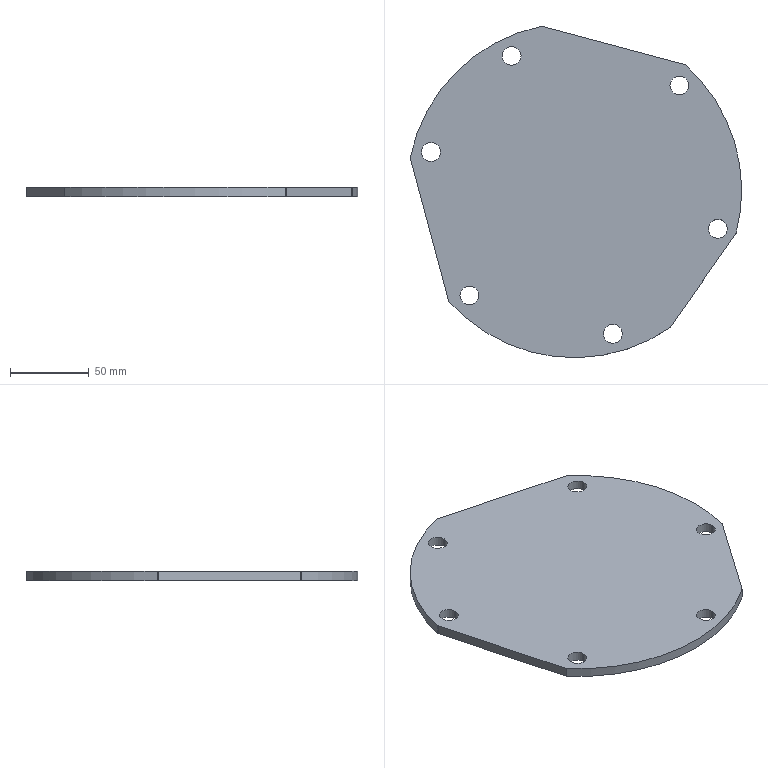Part | SolidWorks | features FlatPattern 1, SMBaseFlange 1, SheetMetal 1 | 1 solid | 27 faces | box 210.92 x 210.92 x 6 mm | volume 199422 mm3 | cylinder 22 | plane 5 | commonest cylinder face diameters 12 x12 2 x7 213 x3
STEP:
#1=CARTESIAN_POINT('',(18.458,-91.28,6.));
#2=VERTEX_POINT('',#1);
#3=CARTESIAN_POINT('',(30.458,-91.28,6.));
#4=VERTEX_POINT('',#3);
#5=CARTESIAN_POINT('',(24.458,-91.28,6.));
#6=DIRECTION('',(0.,0.,1.));
#7=DIRECTION('',(1.,0.,0.));
#8=AXIS2_PLACEMENT_3D('',#5,#6,#7);
#9=CIRCLE('',#8,6.);
#10=EDGE_CURVE('',#2,#4,#9,.T.);
#11=ORIENTED_EDGE('',*,*,#10,.T.);
#12=CARTESIAN_POINT('',(30.458,-91.28,0.));
#13=VERTEX_POINT('',#12);
#14=CARTESIAN_POINT('',(30.458,-91.28,6.));
#15=DIRECTION('',(0.,0.,-1.));
#16=VECTOR('',#15,1000.);
#17=LINE('',#14,#16);
#18=EDGE_CURVE('',#4,#13,#17,.T.);
#19=ORIENTED_EDGE('',*,*,#18,.T.);
#20=CARTESIAN_POINT('',(18.458,-91.28,0.));
#21=VERTEX_POINT('',#20);
#22=CARTESIAN_POINT('',(24.458,-91.28,0.));
#23=DIRECTION('',(0.,0.,1.));
#24=DIRECTION('',(1.,0.,0.));
#25=AXIS2_PLACEMENT_3D('',#22,#23,#24);
#26=CIRCLE('',#25,6.);
#27=EDGE_CURVE('',#21,#13,#26,.T.);
#28=ORIENTED_EDGE('',*,*,#27,.F.);
#29=CARTESIAN_POINT('',(18.458,-91.28,6.));
#30=DIRECTION('',(0.,0.,-1.));
#31=VECTOR('',#30,1000.);
#32=LINE('',#29,#31);
#33=EDGE_CURVE('',#2,#21,#32,.T.);
#34=ORIENTED_EDGE('',*,*,#33,.F.);
#35=EDGE_LOOP('',(#11,#19,#28,#34));
#36=FACE_OUTER_BOUND('',#35,.T.);
#37=CARTESIAN_POINT('',(24.458,-91.28,6.));
#38=DIRECTION('',(0.,0.,-1.));
#39=DIRECTION('',(-1.,0.,0.));
#40=AXIS2_PLACEMENT_3D('',#37,#38,#39);
#41=CYLINDRICAL_SURFACE('',#40,6.);
#42=ADVANCED_FACE('',(#36),#41,.F.);
#43=CARTESIAN_POINT('',(85.28,-24.458,6.));
#44=VERTEX_POINT('',#43);
#45=CARTESIAN_POINT('',(97.28,-24.458,6.));
#46=VERTEX_POINT('',#45);
#47=CARTESIAN_POINT('',(91.28,-24.458,6.));
#48=DIRECTION('',(0.,0.,1.));
#49=DIRECTION('',(1.,0.,0.));
#50=AXIS2_PLACEMENT_3D('',#47,#48,#49);
#51=CIRCLE('',#50,6.);
#52=EDGE_CURVE('',#44,#46,#51,.T.);
#53=ORIENTED_EDGE('',*,*,#52,.T.);
#54=CARTESIAN_POINT('',(97.28,-24.458,0.));
#55=VERTEX_POINT('',#54);
#56=CARTESIAN_POINT('',(97.28,-24.458,6.));
#57=DIRECTION('',(0.,0.,-1.));
#58=VECTOR('',#57,1000.);
#59=LINE('',#56,#58);
#60=EDGE_CURVE('',#46,#55,#59,.T.);
#61=ORIENTED_EDGE('',*,*,#60,.T.);
#62=CARTESIAN_POINT('',(85.28,-24.458,0.));
#63=VERTEX_POINT('',#62);
#64=CARTESIAN_POINT('',(91.28,-24.458,0.));
#65=DIRECTION('',(0.,0.,1.));
#66=DIRECTION('',(1.,0.,0.));
#67=AXIS2_PLACEMENT_3D('',#64,#65,#66);
#68=CIRCLE('',#67,6.);
#69=EDGE_CURVE('',#63,#55,#68,.T.);
#70=ORIENTED_EDGE('',*,*,#69,.F.);
#71=CARTESIAN_POINT('',(85.28,-24.458,6.));
#72=DIRECTION('',(0.,0.,-1.));
#73=VECTOR('',#72,1000.);
#74=LINE('',#71,#73);
#75=EDGE_CURVE('',#44,#63,#74,.T.);
#76=ORIENTED_EDGE('',*,*,#75,.F.);
#77=EDGE_LOOP('',(#53,#61,#70,#76));
#78=FACE_OUTER_BOUND('',#77,.T.);
#79=CARTESIAN_POINT('',(91.28,-24.458,6.));
#80=DIRECTION('',(0.,0.,-1.));
#81=DIRECTION('',(-1.,0.,0.));
#82=AXIS2_PLACEMENT_3D('',#79,#80,#81);
#83=CYLINDRICAL_SURFACE('',#82,6.);
#84=ADVANCED_FACE('',(#78),#83,.F.);
#85=CARTESIAN_POINT('',(60.822,66.822,6.));
#86=VERTEX_POINT('',#85);
#87=CARTESIAN_POINT('',(72.822,66.822,6.));
#88=VERTEX_POINT('',#87);
#89=CARTESIAN_POINT('',(66.822,66.822,6.));
#90=DIRECTION('',(0.,0.,1.));
#91=DIRECTION('',(1.,0.,0.));
#92=AXIS2_PLACEMENT_3D('',#89,#90,#91);
#93=CIRCLE('',#92,6.);
#94=EDGE_CURVE('',#86,#88,#93,.T.);
#95=ORIENTED_EDGE('',*,*,#94,.T.);
#96=CARTESIAN_POINT('',(72.822,66.822,0.));
#97=VERTEX_POINT('',#96);
#98=CARTESIAN_POINT('',(72.822,66.822,6.));
#99=DIRECTION('',(0.,0.,-1.));
#100=VECTOR('',#99,1000.);
#101=LINE('',#98,#100);
#102=EDGE_CURVE('',#88,#97,#101,.T.);
#103=ORIENTED_EDGE('',*,*,#102,.T.);
#104=CARTESIAN_POINT('',(60.822,66.822,0.));
#105=VERTEX_POINT('',#104);
#106=CARTESIAN_POINT('',(66.822,66.822,0.));
#107=DIRECTION('',(0.,0.,1.));
#108=DIRECTION('',(1.,0.,0.));
#109=AXIS2_PLACEMENT_3D('',#106,#107,#108);
#110=CIRCLE('',#109,6.);
#111=EDGE_CURVE('',#105,#97,#110,.T.);
#112=ORIENTED_EDGE('',*,*,#111,.F.);
#113=CARTESIAN_POINT('',(60.822,66.822,6.));
#114=DIRECTION('',(0.,0.,-1.));
#115=VECTOR('',#114,1000.);
#116=LINE('',#113,#115);
#117=EDGE_CURVE('',#86,#105,#116,.T.);
#118=ORIENTED_EDGE('',*,*,#117,.F.);
#119=EDGE_LOOP('',(#95,#103,#112,#118));
#120=FACE_OUTER_BOUND('',#119,.T.);
#121=CARTESIAN_POINT('',(66.822,66.822,6.));
#122=DIRECTION('',(0.,0.,-1.));
#123=DIRECTION('',(-1.,0.,0.));
#124=AXIS2_PLACEMENT_3D('',#121,#122,#123);
#125=CYLINDRICAL_SURFACE('',#124,6.);
#126=ADVANCED_FACE('',(#120),#125,.F.);
#127=CARTESIAN_POINT('',(-45.937,85.646,6.));
#128=VERTEX_POINT('',#127);
#129=CARTESIAN_POINT('',(-33.937,85.646,6.));
#130=VERTEX_POINT('',#129);
#131=CARTESIAN_POINT('',(-39.937,85.646,6.));
#132=DIRECTION('',(0.,0.,1.));
#133=DIRECTION('',(1.,0.,0.));
#134=AXIS2_PLACEMENT_3D('',#131,#132,#133);
#135=CIRCLE('',#134,6.);
#136=EDGE_CURVE('',#128,#130,#135,.T.);
#137=ORIENTED_EDGE('',*,*,#136,.T.);
#138=CARTESIAN_POINT('',(-33.937,85.646,0.));
#139=VERTEX_POINT('',#138);
#140=CARTESIAN_POINT('',(-33.937,85.646,6.));
#141=DIRECTION('',(0.,0.,-1.));
#142=VECTOR('',#141,1000.);
#143=LINE('',#140,#142);
#144=EDGE_CURVE('',#130,#139,#143,.T.);
#145=ORIENTED_EDGE('',*,*,#144,.T.);
#146=CARTESIAN_POINT('',(-45.937,85.646,0.));
#147=VERTEX_POINT('',#146);
#148=CARTESIAN_POINT('',(-39.937,85.646,0.));
#149=DIRECTION('',(0.,0.,1.));
#150=DIRECTION('',(1.,0.,0.));
#151=AXIS2_PLACEMENT_3D('',#148,#149,#150);
#152=CIRCLE('',#151,6.);
#153=EDGE_CURVE('',#147,#139,#152,.T.);
#154=ORIENTED_EDGE('',*,*,#153,.F.);
#155=CARTESIAN_POINT('',(-45.937,85.646,6.));
#156=DIRECTION('',(0.,0.,-1.));
#157=VECTOR('',#156,1000.);
#158=LINE('',#155,#157);
#159=EDGE_CURVE('',#128,#147,#158,.T.);
#160=ORIENTED_EDGE('',*,*,#159,.F.);
#161=EDGE_LOOP('',(#137,#145,#154,#160));
#162=FACE_OUTER_BOUND('',#161,.T.);
#163=CARTESIAN_POINT('',(-39.937,85.646,6.));
#164=DIRECTION('',(0.,0.,-1.));
#165=DIRECTION('',(-1.,0.,0.));
#166=AXIS2_PLACEMENT_3D('',#163,#164,#165);
#167=CYLINDRICAL_SURFACE('',#166,6.);
#168=ADVANCED_FACE('',(#162),#167,.F.);
#169=CARTESIAN_POINT('',(-97.28,24.458,6.));
#170=VERTEX_POINT('',#169);
#171=CARTESIAN_POINT('',(-85.28,24.458,6.));
#172=VERTEX_POINT('',#171);
#173=CARTESIAN_POINT('',(-91.28,24.458,6.));
#174=DIRECTION('',(0.,0.,1.));
#175=DIRECTION('',(1.,0.,0.));
#176=AXIS2_PLACEMENT_3D('',#173,#174,#175);
#177=CIRCLE('',#176,6.);
#178=EDGE_CURVE('',#170,#172,#177,.T.);
#179=ORIENTED_EDGE('',*,*,#178,.T.);
#180=CARTESIAN_POINT('',(-85.28,24.458,0.));
#181=VERTEX_POINT('',#180);
#182=CARTESIAN_POINT('',(-85.28,24.458,6.));
#183=DIRECTION('',(0.,0.,-1.));
#184=VECTOR('',#183,1000.);
#185=LINE('',#182,#184);
#186=EDGE_CURVE('',#172,#181,#185,.T.);
#187=ORIENTED_EDGE('',*,*,#186,.T.);
#188=CARTESIAN_POINT('',(-97.28,24.458,0.));
#189=VERTEX_POINT('',#188);
#190=CARTESIAN_POINT('',(-91.28,24.458,0.));
#191=DIRECTION('',(0.,0.,1.));
#192=DIRECTION('',(1.,0.,0.));
#193=AXIS2_PLACEMENT_3D('',#190,#191,#192);
#194=CIRCLE('',#193,6.);
#195=EDGE_CURVE('',#189,#181,#194,.T.);
#196=ORIENTED_EDGE('',*,*,#195,.F.);
#197=CARTESIAN_POINT('',(-97.28,24.458,6.));
#198=DIRECTION('',(0.,0.,-1.));
#199=VECTOR('',#198,1000.);
#200=LINE('',#197,#199);
#201=EDGE_CURVE('',#170,#189,#200,.T.);
#202=ORIENTED_EDGE('',*,*,#201,.F.);
#203=EDGE_LOOP('',(#179,#187,#196,#202));
#204=FACE_OUTER_BOUND('',#203,.T.);
#205=CARTESIAN_POINT('',(-91.28,24.458,6.));
#206=DIRECTION('',(0.,0.,-1.));
#207=DIRECTION('',(-1.,0.,0.));
#208=AXIS2_PLACEMENT_3D('',#205,#206,#207);
#209=CYLINDRICAL_SURFACE('',#208,6.);
#210=ADVANCED_FACE('',(#204),#209,.F.);
#211=CARTESIAN_POINT('',(-72.822,-66.822,6.));
#212=VERTEX_POINT('',#211);
#213=CARTESIAN_POINT('',(-60.822,-66.822,6.));
#214=VERTEX_POINT('',#213);
#215=CARTESIAN_POINT('',(-66.822,-66.822,6.));
#216=DIRECTION('',(0.,0.,1.));
#217=DIRECTION('',(1.,0.,0.));
#218=AXIS2_PLACEMENT_3D('',#215,#216,#217);
#219=CIRCLE('',#218,6.);
#220=EDGE_CURVE('',#212,#214,#219,.T.);
#221=ORIENTED_EDGE('',*,*,#220,.T.);
#222=CARTESIAN_POINT('',(-60.822,-66.822,0.));
#223=VERTEX_POINT('',#222);
#224=CARTESIAN_POINT('',(-60.822,-66.822,6.));
#225=DIRECTION('',(0.,0.,-1.));
#226=VECTOR('',#225,1000.);
#227=LINE('',#224,#226);
#228=EDGE_CURVE('',#214,#223,#227,.T.);
#229=ORIENTED_EDGE('',*,*,#228,.T.);
#230=CARTESIAN_POINT('',(-72.822,-66.822,0.));
#231=VERTEX_POINT('',#230);
#232=CARTESIAN_POINT('',(-66.822,-66.822,0.));
#233=DIRECTION('',(0.,0.,1.));
#234=DIRECTION('',(1.,0.,0.));
#235=AXIS2_PLACEMENT_3D('',#232,#233,#234);
#236=CIRCLE('',#235,6.);
#237=EDGE_CURVE('',#231,#223,#236,.T.);
#238=ORIENTED_EDGE('',*,*,#237,.F.);
#239=CARTESIAN_POINT('',(-72.822,-66.822,6.));
#240=DIRECTION('',(0.,0.,-1.));
#241=VECTOR('',#240,1000.);
#242=LINE('',#239,#241);
#243=EDGE_CURVE('',#212,#231,#242,.T.);
#244=ORIENTED_EDGE('',*,*,#243,.F.);
#245=EDGE_LOOP('',(#221,#229,#238,#244));
#246=FACE_OUTER_BOUND('',#245,.T.);
#247=CARTESIAN_POINT('',(-66.822,-66.822,6.));
#248=DIRECTION('',(0.,0.,-1.));
#249=DIRECTION('',(-1.,0.,0.));
#250=AXIS2_PLACEMENT_3D('',#247,#248,#249);
#251=CYLINDRICAL_SURFACE('',#250,6.);
#252=ADVANCED_FACE('',(#246),#251,.F.);
#253=CARTESIAN_POINT('',(-104.42,20.848,6.));
#254=VERTEX_POINT('',#253);
#255=CARTESIAN_POINT('',(-104.386,20.589,6.));
#256=VERTEX_POINT('',#255);
#257=CARTESIAN_POINT('',(-103.42,20.848,6.));
#258=DIRECTION('',(0.,0.,1.));
#259=DIRECTION('',(1.,0.,0.));
#260=AXIS2_PLACEMENT_3D('',#257,#258,#259);
#261=CIRCLE('',#260,1.);
#262=EDGE_CURVE('',#254,#256,#261,.T.);
#263=ORIENTED_EDGE('',*,*,#262,.F.);
#264=CARTESIAN_POINT('',(-104.42,20.848,0.));
#265=VERTEX_POINT('',#264);
#266=CARTESIAN_POINT('',(-104.42,20.848,6.));
#267=DIRECTION('',(0.,0.,-1.));
#268=VECTOR('',#267,1000.);
#269=LINE('',#266,#268);
#270=EDGE_CURVE('',#254,#265,#269,.T.);
#271=ORIENTED_EDGE('',*,*,#270,.T.);
#272=CARTESIAN_POINT('',(-104.386,20.589,0.));
#273=VERTEX_POINT('',#272);
#274=CARTESIAN_POINT('',(-103.42,20.848,0.));
#275=DIRECTION('',(0.,0.,1.));
#276=DIRECTION('',(1.,0.,0.));
#277=AXIS2_PLACEMENT_3D('',#274,#275,#276);
#278=CIRCLE('',#277,1.);
#279=EDGE_CURVE('',#265,#273,#278,.T.);
#280=ORIENTED_EDGE('',*,*,#279,.T.);
#281=CARTESIAN_POINT('',(-104.386,20.589,6.));
#282=DIRECTION('',(0.,0.,-1.));
#283=VECTOR('',#282,1000.);
#284=LINE('',#281,#283);
#285=EDGE_CURVE('',#256,#273,#284,.T.);
#286=ORIENTED_EDGE('',*,*,#285,.F.);
#287=EDGE_LOOP('',(#263,#271,#280,#286));
#288=FACE_OUTER_BOUND('',#287,.T.);
#289=CARTESIAN_POINT('',(-103.42,20.848,6.));
#290=DIRECTION('',(0.,0.,-1.));
#291=DIRECTION('',(-1.,0.,0.));
#292=AXIS2_PLACEMENT_3D('',#289,#290,#291);
#293=CYLINDRICAL_SURFACE('',#292,1.);
#294=ADVANCED_FACE('',(#288),#293,.T.);
#295=ORIENTED_EDGE('',*,*,#52,.F.);
#296=CARTESIAN_POINT('',(91.28,-24.458,6.));
#297=DIRECTION('',(0.,0.,1.));
#298=DIRECTION('',(1.,0.,0.));
#299=AXIS2_PLACEMENT_3D('',#296,#297,#298);
#300=CIRCLE('',#299,6.);
#301=EDGE_CURVE('',#46,#44,#300,.T.);
#302=ORIENTED_EDGE('',*,*,#301,.F.);
#303=EDGE_LOOP('',(#295,#302));
#304=FACE_BOUND('',#303,.T.);
#305=ORIENTED_EDGE('',*,*,#136,.F.);
#306=CARTESIAN_POINT('',(-39.937,85.646,6.));
#307=DIRECTION('',(0.,0.,1.));
#308=DIRECTION('',(1.,0.,0.));
#309=AXIS2_PLACEMENT_3D('',#306,#307,#308);
#310=CIRCLE('',#309,6.);
#311=EDGE_CURVE('',#130,#128,#310,.T.);
#312=ORIENTED_EDGE('',*,*,#311,.F.);
#313=EDGE_LOOP('',(#305,#312));
#314=FACE_BOUND('',#313,.T.);
#315=ORIENTED_EDGE('',*,*,#220,.F.);
#316=CARTESIAN_POINT('',(-66.822,-66.822,6.));
#317=DIRECTION('',(0.,0.,1.));
#318=DIRECTION('',(1.,0.,0.));
#319=AXIS2_PLACEMENT_3D('',#316,#317,#318);
#320=CIRCLE('',#319,6.);
#321=EDGE_CURVE('',#214,#212,#320,.T.);
#322=ORIENTED_EDGE('',*,*,#321,.F.);
#323=EDGE_LOOP('',(#315,#322));
#324=FACE_BOUND('',#323,.T.);
#325=CARTESIAN_POINT('',(60.755,-87.471,6.));
#326=VERTEX_POINT('',#325);
#327=CARTESIAN_POINT('',(61.003,-87.223,6.));
#328=VERTEX_POINT('',#327);
#329=CARTESIAN_POINT('',(60.184,-86.649,6.));
#330=DIRECTION('',(0.,0.,1.));
#331=DIRECTION('',(1.,0.,0.));
#332=AXIS2_PLACEMENT_3D('',#329,#330,#331);
#333=CIRCLE('',#332,1.);
#334=EDGE_CURVE('',#326,#328,#333,.T.);
#335=ORIENTED_EDGE('',*,*,#334,.T.);
#336=CARTESIAN_POINT('',(102.827,-27.492,6.));
#337=VERTEX_POINT('',#336);
#338=CARTESIAN_POINT('',(61.003,-87.223,6.));
#339=DIRECTION('',(0.5736,0.8192,0.));
#340=VECTOR('',#339,1000.);
#341=LINE('',#338,#340);
#342=EDGE_CURVE('',#328,#337,#341,.T.);
#343=ORIENTED_EDGE('',*,*,#342,.T.);
#344=CARTESIAN_POINT('',(102.975,-27.174,6.));
#345=VERTEX_POINT('',#344);
#346=CARTESIAN_POINT('',(102.008,-26.919,6.));
#347=DIRECTION('',(0.,0.,1.));
#348=DIRECTION('',(1.,0.,0.));
#349=AXIS2_PLACEMENT_3D('',#346,#347,#348);
#350=CIRCLE('',#349,1.);
#351=EDGE_CURVE('',#337,#345,#350,.T.);
#352=ORIENTED_EDGE('',*,*,#351,.T.);
#353=CARTESIAN_POINT('',(70.426,79.89,6.));
#354=VERTEX_POINT('',#353);
#355=CARTESIAN_POINT('',(0.,0.,6.));
#356=DIRECTION('',(0.,0.,1.));
#357=DIRECTION('',(1.,0.,0.));
#358=AXIS2_PLACEMENT_3D('',#355,#356,#357);
#359=CIRCLE('',#358,106.5);
#360=EDGE_CURVE('',#345,#354,#359,.T.);
#361=ORIENTED_EDGE('',*,*,#360,.T.);
#362=CARTESIAN_POINT('',(70.023,80.106,6.));
#363=VERTEX_POINT('',#362);
#364=CARTESIAN_POINT('',(69.764,79.14,6.));
#365=DIRECTION('',(0.,0.,1.));
#366=DIRECTION('',(1.,0.,0.));
#367=AXIS2_PLACEMENT_3D('',#364,#365,#366);
#368=CIRCLE('',#367,1.);
#369=EDGE_CURVE('',#354,#363,#368,.T.);
#370=ORIENTED_EDGE('',*,*,#369,.T.);
#371=CARTESIAN_POINT('',(-20.589,104.386,6.));
#372=VERTEX_POINT('',#371);
#373=CARTESIAN_POINT('',(70.023,80.106,6.));
#374=DIRECTION('',(-0.9659,0.2588,0.));
#375=VECTOR('',#374,1000.);
#376=LINE('',#373,#375);
#377=EDGE_CURVE('',#363,#372,#376,.T.);
#378=ORIENTED_EDGE('',*,*,#377,.T.);
#379=CARTESIAN_POINT('',(-21.045,104.4,6.));
#380=VERTEX_POINT('',#379);
#381=CARTESIAN_POINT('',(-20.848,103.42,6.));
#382=DIRECTION('',(0.,0.,1.));
#383=DIRECTION('',(1.,0.,0.));
#384=AXIS2_PLACEMENT_3D('',#381,#382,#383);
#385=CIRCLE('',#384,1.);
#386=EDGE_CURVE('',#372,#380,#385,.T.);
#387=ORIENTED_EDGE('',*,*,#386,.T.);
#388=CARTESIAN_POINT('',(-104.4,21.045,6.));
#389=VERTEX_POINT('',#388);
#390=CARTESIAN_POINT('',(0.,0.,6.));
#391=DIRECTION('',(0.,0.,1.));
#392=DIRECTION('',(1.,0.,0.));
#393=AXIS2_PLACEMENT_3D('',#390,#391,#392);
#394=CIRCLE('',#393,106.5);
#395=EDGE_CURVE('',#380,#389,#394,.T.);
#396=ORIENTED_EDGE('',*,*,#395,.T.);
#397=CARTESIAN_POINT('',(-103.42,20.848,6.));
#398=DIRECTION('',(0.,0.,1.));
#399=DIRECTION('',(1.,0.,0.));
#400=AXIS2_PLACEMENT_3D('',#397,#398,#399);
#401=CIRCLE('',#400,1.);
#402=EDGE_CURVE('',#389,#254,#401,.T.);
#403=ORIENTED_EDGE('',*,*,#402,.T.);
#404=ORIENTED_EDGE('',*,*,#262,.T.);
#405=CARTESIAN_POINT('',(-80.106,-70.023,6.));
#406=VERTEX_POINT('',#405);
#407=CARTESIAN_POINT('',(-104.386,20.589,6.));
#408=DIRECTION('',(0.2588,-0.9659,0.));
#409=VECTOR('',#408,1000.);
#410=LINE('',#407,#409);
#411=EDGE_CURVE('',#256,#406,#410,.T.);
#412=ORIENTED_EDGE('',*,*,#411,.T.);
#413=CARTESIAN_POINT('',(-79.89,-70.426,6.));
#414=VERTEX_POINT('',#413);
#415=CARTESIAN_POINT('',(-79.14,-69.764,6.));
#416=DIRECTION('',(0.,0.,1.));
#417=DIRECTION('',(1.,0.,0.));
#418=AXIS2_PLACEMENT_3D('',#415,#416,#417);
#419=CIRCLE('',#418,1.);
#420=EDGE_CURVE('',#406,#414,#419,.T.);
#421=ORIENTED_EDGE('',*,*,#420,.T.);
#422=CARTESIAN_POINT('',(0.,0.,6.));
#423=DIRECTION('',(0.,0.,1.));
#424=DIRECTION('',(1.,0.,0.));
#425=AXIS2_PLACEMENT_3D('',#422,#423,#424);
#426=CIRCLE('',#425,106.5);
#427=EDGE_CURVE('',#414,#326,#426,.T.);
#428=ORIENTED_EDGE('',*,*,#427,.T.);
#429=EDGE_LOOP('',(#335,#343,#352,#361,#370,#378,#387,#396,#403,#404,#412,#421,#428));
#430=FACE_OUTER_BOUND('',#429,.T.);
#431=ORIENTED_EDGE('',*,*,#178,.F.);
#432=CARTESIAN_POINT('',(-91.28,24.458,6.));
#433=DIRECTION('',(0.,0.,1.));
#434=DIRECTION('',(1.,0.,0.));
#435=AXIS2_PLACEMENT_3D('',#432,#433,#434);
#436=CIRCLE('',#435,6.);
#437=EDGE_CURVE('',#172,#170,#436,.T.);
#438=ORIENTED_EDGE('',*,*,#437,.F.);
#439=EDGE_LOOP('',(#431,#438));
#440=FACE_BOUND('',#439,.T.);
#441=ORIENTED_EDGE('',*,*,#94,.F.);
#442=CARTESIAN_POINT('',(66.822,66.822,6.));
#443=DIRECTION('',(0.,0.,1.));
#444=DIRECTION('',(1.,0.,0.));
#445=AXIS2_PLACEMENT_3D('',#442,#443,#444);
#446=CIRCLE('',#445,6.);
#447=EDGE_CURVE('',#88,#86,#446,.T.);
#448=ORIENTED_EDGE('',*,*,#447,.F.);
#449=EDGE_LOOP('',(#441,#448));
#450=FACE_BOUND('',#449,.T.);
#451=ORIENTED_EDGE('',*,*,#10,.F.);
#452=CARTESIAN_POINT('',(24.458,-91.28,6.));
#453=DIRECTION('',(0.,0.,1.));
#454=DIRECTION('',(1.,0.,0.));
#455=AXIS2_PLACEMENT_3D('',#452,#453,#454);
#456=CIRCLE('',#455,6.);
#457=EDGE_CURVE('',#4,#2,#456,.T.);
#458=ORIENTED_EDGE('',*,*,#457,.F.);
#459=EDGE_LOOP('',(#451,#458));
#460=FACE_BOUND('',#459,.T.);
#461=CARTESIAN_POINT('',(60.184,-86.649,6.));
#462=DIRECTION('',(0.,0.,1.));
#463=DIRECTION('',(1.,0.,0.));
#464=AXIS2_PLACEMENT_3D('',#461,#462,#463);
#465=PLANE('',#464);
#466=ADVANCED_FACE('',(#304,#314,#324,#430,#440,#450,#460),#465,.T.);
#467=CARTESIAN_POINT('',(60.755,-87.471,0.));
#468=VERTEX_POINT('',#467);
#469=CARTESIAN_POINT('',(61.003,-87.223,0.));
#470=VERTEX_POINT('',#469);
#471=CARTESIAN_POINT('',(60.184,-86.649,0.));
#472=DIRECTION('',(0.,0.,1.));
#473=DIRECTION('',(1.,0.,0.));
#474=AXIS2_PLACEMENT_3D('',#471,#472,#473);
#475=CIRCLE('',#474,1.);
#476=EDGE_CURVE('',#468,#470,#475,.T.);
#477=ORIENTED_EDGE('',*,*,#476,.F.);
#478=CARTESIAN_POINT('',(-79.89,-70.426,0.));
#479=VERTEX_POINT('',#478);
#480=CARTESIAN_POINT('',(0.,0.,0.));
#481=DIRECTION('',(0.,0.,1.));
#482=DIRECTION('',(1.,0.,0.));
#483=AXIS2_PLACEMENT_3D('',#480,#481,#482);
#484=CIRCLE('',#483,106.5);
#485=EDGE_CURVE('',#479,#468,#484,.T.);
#486=ORIENTED_EDGE('',*,*,#485,.F.);
#487=CARTESIAN_POINT('',(-80.106,-70.023,0.));
#488=VERTEX_POINT('',#487);
#489=CARTESIAN_POINT('',(-79.14,-69.764,0.));
#490=DIRECTION('',(0.,0.,1.));
#491=DIRECTION('',(1.,0.,0.));
#492=AXIS2_PLACEMENT_3D('',#489,#490,#491);
#493=CIRCLE('',#492,1.);
#494=EDGE_CURVE('',#488,#479,#493,.T.);
#495=ORIENTED_EDGE('',*,*,#494,.F.);
#496=CARTESIAN_POINT('',(-104.386,20.589,0.));
#497=DIRECTION('',(0.2588,-0.9659,0.));
#498=VECTOR('',#497,1000.);
#499=LINE('',#496,#498);
#500=EDGE_CURVE('',#273,#488,#499,.T.);
#501=ORIENTED_EDGE('',*,*,#500,.F.);
#502=ORIENTED_EDGE('',*,*,#279,.F.);
#503=CARTESIAN_POINT('',(-104.4,21.045,0.));
#504=VERTEX_POINT('',#503);
#505=CARTESIAN_POINT('',(-103.42,20.848,0.));
#506=DIRECTION('',(0.,0.,1.));
#507=DIRECTION('',(1.,0.,0.));
#508=AXIS2_PLACEMENT_3D('',#505,#506,#507);
#509=CIRCLE('',#508,1.);
#510=EDGE_CURVE('',#504,#265,#509,.T.);
#511=ORIENTED_EDGE('',*,*,#510,.F.);
#512=CARTESIAN_POINT('',(-21.045,104.4,0.));
#513=VERTEX_POINT('',#512);
#514=CARTESIAN_POINT('',(0.,0.,0.));
#515=DIRECTION('',(0.,0.,1.));
#516=DIRECTION('',(1.,0.,0.));
#517=AXIS2_PLACEMENT_3D('',#514,#515,#516);
#518=CIRCLE('',#517,106.5);
#519=EDGE_CURVE('',#513,#504,#518,.T.);
#520=ORIENTED_EDGE('',*,*,#519,.F.);
#521=CARTESIAN_POINT('',(-20.589,104.386,0.));
#522=VERTEX_POINT('',#521);
#523=CARTESIAN_POINT('',(-20.848,103.42,0.));
#524=DIRECTION('',(0.,0.,1.));
#525=DIRECTION('',(1.,0.,0.));
#526=AXIS2_PLACEMENT_3D('',#523,#524,#525);
#527=CIRCLE('',#526,1.);
#528=EDGE_CURVE('',#522,#513,#527,.T.);
#529=ORIENTED_EDGE('',*,*,#528,.F.);
#530=CARTESIAN_POINT('',(70.023,80.106,0.));
#531=VERTEX_POINT('',#530);
#532=CARTESIAN_POINT('',(70.023,80.106,0.));
#533=DIRECTION('',(-0.9659,0.2588,0.));
#534=VECTOR('',#533,1000.);
#535=LINE('',#532,#534);
#536=EDGE_CURVE('',#531,#522,#535,.T.);
#537=ORIENTED_EDGE('',*,*,#536,.F.);
#538=CARTESIAN_POINT('',(70.426,79.89,0.));
#539=VERTEX_POINT('',#538);
#540=CARTESIAN_POINT('',(69.764,79.14,0.));
#541=DIRECTION('',(0.,0.,1.));
#542=DIRECTION('',(1.,0.,0.));
#543=AXIS2_PLACEMENT_3D('',#540,#541,#542);
#544=CIRCLE('',#543,1.);
#545=EDGE_CURVE('',#539,#531,#544,.T.);
#546=ORIENTED_EDGE('',*,*,#545,.F.);
#547=CARTESIAN_POINT('',(102.975,-27.174,0.));
#548=VERTEX_POINT('',#547);
#549=CARTESIAN_POINT('',(0.,0.,0.));
#550=DIRECTION('',(0.,0.,1.));
#551=DIRECTION('',(1.,0.,0.));
#552=AXIS2_PLACEMENT_3D('',#549,#550,#551);
#553=CIRCLE('',#552,106.5);
#554=EDGE_CURVE('',#548,#539,#553,.T.);
#555=ORIENTED_EDGE('',*,*,#554,.F.);
#556=CARTESIAN_POINT('',(102.827,-27.492,0.));
#557=VERTEX_POINT('',#556);
#558=CARTESIAN_POINT('',(102.008,-26.919,0.));
#559=DIRECTION('',(0.,0.,1.));
#560=DIRECTION('',(1.,0.,0.));
#561=AXIS2_PLACEMENT_3D('',#558,#559,#560);
#562=CIRCLE('',#561,1.);
#563=EDGE_CURVE('',#557,#548,#562,.T.);
#564=ORIENTED_EDGE('',*,*,#563,.F.);
#565=CARTESIAN_POINT('',(61.003,-87.223,0.));
#566=DIRECTION('',(0.5736,0.8192,0.));
#567=VECTOR('',#566,1000.);
#568=LINE('',#565,#567);
#569=EDGE_CURVE('',#470,#557,#568,.T.);
#570=ORIENTED_EDGE('',*,*,#569,.F.);
#571=EDGE_LOOP('',(#477,#486,#495,#501,#502,#511,#520,#529,#537,#546,#555,#564,#570));
#572=FACE_OUTER_BOUND('',#571,.T.);
#573=ORIENTED_EDGE('',*,*,#237,.T.);
#574=CARTESIAN_POINT('',(-66.822,-66.822,0.));
#575=DIRECTION('',(0.,0.,1.));
#576=DIRECTION('',(1.,0.,0.));
#577=AXIS2_PLACEMENT_3D('',#574,#575,#576);
#578=CIRCLE('',#577,6.);
#579=EDGE_CURVE('',#223,#231,#578,.T.);
#580=ORIENTED_EDGE('',*,*,#579,.T.);
#581=EDGE_LOOP('',(#573,#580));
#582=FACE_BOUND('',#581,.T.);
#583=ORIENTED_EDGE('',*,*,#195,.T.);
#584=CARTESIAN_POINT('',(-91.28,24.458,0.));
#585=DIRECTION('',(0.,0.,1.));
#586=DIRECTION('',(1.,0.,0.));
#587=AXIS2_PLACEMENT_3D('',#584,#585,#586);
#588=CIRCLE('',#587,6.);
#589=EDGE_CURVE('',#181,#189,#588,.T.);
#590=ORIENTED_EDGE('',*,*,#589,.T.);
#591=EDGE_LOOP('',(#583,#590));
#592=FACE_BOUND('',#591,.T.);
#593=ORIENTED_EDGE('',*,*,#153,.T.);
#594=CARTESIAN_POINT('',(-39.937,85.646,0.));
#595=DIRECTION('',(0.,0.,1.));
#596=DIRECTION('',(1.,0.,0.));
#597=AXIS2_PLACEMENT_3D('',#594,#595,#596);
#598=CIRCLE('',#597,6.);
#599=EDGE_CURVE('',#139,#147,#598,.T.);
#600=ORIENTED_EDGE('',*,*,#599,.T.);
#601=EDGE_LOOP('',(#593,#600));
#602=FACE_BOUND('',#601,.T.);
#603=ORIENTED_EDGE('',*,*,#111,.T.);
#604=CARTESIAN_POINT('',(66.822,66.822,0.));
#605=DIRECTION('',(0.,0.,1.));
#606=DIRECTION('',(1.,0.,0.));
#607=AXIS2_PLACEMENT_3D('',#604,#605,#606);
#608=CIRCLE('',#607,6.);
#609=EDGE_CURVE('',#97,#105,#608,.T.);
#610=ORIENTED_EDGE('',*,*,#609,.T.);
#611=EDGE_LOOP('',(#603,#610));
#612=FACE_BOUND('',#611,.T.);
#613=ORIENTED_EDGE('',*,*,#69,.T.);
#614=CARTESIAN_POINT('',(91.28,-24.458,0.));
#615=DIRECTION('',(0.,0.,1.));
#616=DIRECTION('',(1.,0.,0.));
#617=AXIS2_PLACEMENT_3D('',#614,#615,#616);
#618=CIRCLE('',#617,6.);
#619=EDGE_CURVE('',#55,#63,#618,.T.);
#620=ORIENTED_EDGE('',*,*,#619,.T.);
#621=EDGE_LOOP('',(#613,#620));
#622=FACE_BOUND('',#621,.T.);
#623=ORIENTED_EDGE('',*,*,#27,.T.);
#624=CARTESIAN_POINT('',(24.458,-91.28,0.));
#625=DIRECTION('',(0.,0.,1.));
#626=DIRECTION('',(1.,0.,0.));
#627=AXIS2_PLACEMENT_3D('',#624,#625,#626);
#628=CIRCLE('',#627,6.);
#629=EDGE_CURVE('',#13,#21,#628,.T.);
#630=ORIENTED_EDGE('',*,*,#629,.T.);
#631=EDGE_LOOP('',(#623,#630));
#632=FACE_BOUND('',#631,.T.);
#633=CARTESIAN_POINT('',(60.184,-86.649,0.));
#634=DIRECTION('',(0.,0.,1.));
#635=DIRECTION('',(1.,0.,0.));
#636=AXIS2_PLACEMENT_3D('',#633,#634,#635);
#637=PLANE('',#636);
#638=ADVANCED_FACE('',(#572,#582,#592,#602,#612,#622,#632),#637,.F.);
#639=ORIENTED_EDGE('',*,*,#476,.T.);
#640=CARTESIAN_POINT('',(61.003,-87.223,6.));
#641=DIRECTION('',(0.,0.,-1.));
#642=VECTOR('',#641,1000.);
#643=LINE('',#640,#642);
#644=EDGE_CURVE('',#328,#470,#643,.T.);
#645=ORIENTED_EDGE('',*,*,#644,.F.);
#646=ORIENTED_EDGE('',*,*,#334,.F.);
#647=CARTESIAN_POINT('',(60.755,-87.471,6.));
#648=DIRECTION('',(0.,0.,-1.));
#649=VECTOR('',#648,1000.);
#650=LINE('',#647,#649);
#651=EDGE_CURVE('',#326,#468,#650,.T.);
#652=ORIENTED_EDGE('',*,*,#651,.T.);
#653=EDGE_LOOP('',(#639,#645,#646,#652));
#654=FACE_OUTER_BOUND('',#653,.T.);
#655=CARTESIAN_POINT('',(60.184,-86.649,6.));
#656=DIRECTION('',(0.,0.,-1.));
#657=DIRECTION('',(-1.,0.,0.));
#658=AXIS2_PLACEMENT_3D('',#655,#656,#657);
#659=CYLINDRICAL_SURFACE('',#658,1.);
#660=ADVANCED_FACE('',(#654),#659,.T.);
#661=ORIENTED_EDGE('',*,*,#569,.T.);
#662=CARTESIAN_POINT('',(102.827,-27.492,6.));
#663=DIRECTION('',(0.,0.,-1.));
#664=VECTOR('',#663,1000.);
#665=LINE('',#662,#664);
#666=EDGE_CURVE('',#337,#557,#665,.T.);
#667=ORIENTED_EDGE('',*,*,#666,.F.);
#668=ORIENTED_EDGE('',*,*,#342,.F.);
#669=ORIENTED_EDGE('',*,*,#644,.T.);
#670=EDGE_LOOP('',(#661,#667,#668,#669));
#671=FACE_OUTER_BOUND('',#670,.T.);
#672=CARTESIAN_POINT('',(61.003,-87.223,6.));
#673=DIRECTION('',(-0.8192,0.5736,0.));
#674=DIRECTION('',(-0.5736,-0.8192,0.));
#675=AXIS2_PLACEMENT_3D('',#672,#673,#674);
#676=PLANE('',#675);
#677=ADVANCED_FACE('',(#671),#676,.F.);
#678=ORIENTED_EDGE('',*,*,#563,.T.);
#679=CARTESIAN_POINT('',(102.975,-27.174,6.));
#680=DIRECTION('',(0.,0.,-1.));
#681=VECTOR('',#680,1000.);
#682=LINE('',#679,#681);
#683=EDGE_CURVE('',#345,#548,#682,.T.);
#684=ORIENTED_EDGE('',*,*,#683,.F.);
#685=ORIENTED_EDGE('',*,*,#351,.F.);
#686=ORIENTED_EDGE('',*,*,#666,.T.);
#687=EDGE_LOOP('',(#678,#684,#685,#686));
#688=FACE_OUTER_BOUND('',#687,.T.);
#689=CARTESIAN_POINT('',(102.008,-26.919,6.));
#690=DIRECTION('',(0.,0.,-1.));
#691=DIRECTION('',(-1.,0.,0.));
#692=AXIS2_PLACEMENT_3D('',#689,#690,#691);
#693=CYLINDRICAL_SURFACE('',#692,1.);
#694=ADVANCED_FACE('',(#688),#693,.T.);
#695=ORIENTED_EDGE('',*,*,#554,.T.);
#696=CARTESIAN_POINT('',(70.426,79.89,6.));
#697=DIRECTION('',(0.,0.,-1.));
#698=VECTOR('',#697,1000.);
#699=LINE('',#696,#698);
#700=EDGE_CURVE('',#354,#539,#699,.T.);
#701=ORIENTED_EDGE('',*,*,#700,.F.);
#702=ORIENTED_EDGE('',*,*,#360,.F.);
#703=ORIENTED_EDGE('',*,*,#683,.T.);
#704=EDGE_LOOP('',(#695,#701,#702,#703));
#705=FACE_OUTER_BOUND('',#704,.T.);
#706=CARTESIAN_POINT('',(0.,0.,6.));
#707=DIRECTION('',(0.,0.,-1.));
#708=DIRECTION('',(-1.,0.,0.));
#709=AXIS2_PLACEMENT_3D('',#706,#707,#708);
#710=CYLINDRICAL_SURFACE('',#709,106.5);
#711=ADVANCED_FACE('',(#705),#710,.T.);
#712=ORIENTED_EDGE('',*,*,#545,.T.);
#713=CARTESIAN_POINT('',(70.023,80.106,6.));
#714=DIRECTION('',(0.,0.,-1.));
#715=VECTOR('',#714,1000.);
#716=LINE('',#713,#715);
#717=EDGE_CURVE('',#363,#531,#716,.T.);
#718=ORIENTED_EDGE('',*,*,#717,.F.);
#719=ORIENTED_EDGE('',*,*,#369,.F.);
#720=ORIENTED_EDGE('',*,*,#700,.T.);
#721=EDGE_LOOP('',(#712,#718,#719,#720));
#722=FACE_OUTER_BOUND('',#721,.T.);
#723=CARTESIAN_POINT('',(69.764,79.14,6.));
#724=DIRECTION('',(0.,0.,-1.));
#725=DIRECTION('',(-1.,0.,0.));
#726=AXIS2_PLACEMENT_3D('',#723,#724,#725);
#727=CYLINDRICAL_SURFACE('',#726,1.);
#728=ADVANCED_FACE('',(#722),#727,.T.);
#729=ORIENTED_EDGE('',*,*,#536,.T.);
#730=CARTESIAN_POINT('',(-20.589,104.386,6.));
#731=DIRECTION('',(0.,0.,-1.));
#732=VECTOR('',#731,1000.);
#733=LINE('',#730,#732);
#734=EDGE_CURVE('',#372,#522,#733,.T.);
#735=ORIENTED_EDGE('',*,*,#734,.F.);
#736=ORIENTED_EDGE('',*,*,#377,.F.);
#737=ORIENTED_EDGE('',*,*,#717,.T.);
#738=EDGE_LOOP('',(#729,#735,#736,#737));
#739=FACE_OUTER_BOUND('',#738,.T.);
#740=CARTESIAN_POINT('',(70.023,80.106,6.));
#741=DIRECTION('',(-0.2588,-0.9659,0.));
#742=DIRECTION('',(0.9659,-0.2588,0.));
#743=AXIS2_PLACEMENT_3D('',#740,#741,#742);
#744=PLANE('',#743);
#745=ADVANCED_FACE('',(#739),#744,.F.);
#746=ORIENTED_EDGE('',*,*,#528,.T.);
#747=CARTESIAN_POINT('',(-21.045,104.4,6.));
#748=DIRECTION('',(0.,0.,-1.));
#749=VECTOR('',#748,1000.);
#750=LINE('',#747,#749);
#751=EDGE_CURVE('',#380,#513,#750,.T.);
#752=ORIENTED_EDGE('',*,*,#751,.F.);
#753=ORIENTED_EDGE('',*,*,#386,.F.);
#754=ORIENTED_EDGE('',*,*,#734,.T.);
#755=EDGE_LOOP('',(#746,#752,#753,#754));
#756=FACE_OUTER_BOUND('',#755,.T.);
#757=CARTESIAN_POINT('',(-20.848,103.42,6.));
#758=DIRECTION('',(0.,0.,-1.));
#759=DIRECTION('',(-1.,0.,0.));
#760=AXIS2_PLACEMENT_3D('',#757,#758,#759);
#761=CYLINDRICAL_SURFACE('',#760,1.);
#762=ADVANCED_FACE('',(#756),#761,.T.);
#763=ORIENTED_EDGE('',*,*,#519,.T.);
#764=CARTESIAN_POINT('',(-104.4,21.045,6.));
#765=DIRECTION('',(0.,0.,-1.));
#766=VECTOR('',#765,1000.);
#767=LINE('',#764,#766);
#768=EDGE_CURVE('',#389,#504,#767,.T.);
#769=ORIENTED_EDGE('',*,*,#768,.F.);
#770=ORIENTED_EDGE('',*,*,#395,.F.);
#771=ORIENTED_EDGE('',*,*,#751,.T.);
#772=EDGE_LOOP('',(#763,#769,#770,#771));
#773=FACE_OUTER_BOUND('',#772,.T.);
#774=CARTESIAN_POINT('',(0.,0.,6.));
#775=DIRECTION('',(0.,0.,-1.));
#776=DIRECTION('',(-1.,0.,0.));
#777=AXIS2_PLACEMENT_3D('',#774,#775,#776);
#778=CYLINDRICAL_SURFACE('',#777,106.5);
#779=ADVANCED_FACE('',(#773),#778,.T.);
#780=ORIENTED_EDGE('',*,*,#270,.F.);
#781=ORIENTED_EDGE('',*,*,#402,.F.);
#782=ORIENTED_EDGE('',*,*,#768,.T.);
#783=ORIENTED_EDGE('',*,*,#510,.T.);
#784=EDGE_LOOP('',(#780,#781,#782,#783));
#785=FACE_OUTER_BOUND('',#784,.T.);
#786=CARTESIAN_POINT('',(-103.42,20.848,6.));
#787=DIRECTION('',(0.,0.,-1.));
#788=DIRECTION('',(-1.,0.,0.));
#789=AXIS2_PLACEMENT_3D('',#786,#787,#788);
#790=CYLINDRICAL_SURFACE('',#789,1.);
#791=ADVANCED_FACE('',(#785),#790,.T.);
#792=ORIENTED_EDGE('',*,*,#500,.T.);
#793=CARTESIAN_POINT('',(-80.106,-70.023,6.));
#794=DIRECTION('',(0.,0.,-1.));
#795=VECTOR('',#794,1000.);
#796=LINE('',#793,#795);
#797=EDGE_CURVE('',#406,#488,#796,.T.);
#798=ORIENTED_EDGE('',*,*,#797,.F.);
#799=ORIENTED_EDGE('',*,*,#411,.F.);
#800=ORIENTED_EDGE('',*,*,#285,.T.);
#801=EDGE_LOOP('',(#792,#798,#799,#800));
#802=FACE_OUTER_BOUND('',#801,.T.);
#803=CARTESIAN_POINT('',(-104.386,20.589,6.));
#804=DIRECTION('',(0.9659,0.2588,0.));
#805=DIRECTION('',(-0.2588,0.9659,0.));
#806=AXIS2_PLACEMENT_3D('',#803,#804,#805);
#807=PLANE('',#806);
#808=ADVANCED_FACE('',(#802),#807,.F.);
#809=ORIENTED_EDGE('',*,*,#494,.T.);
#810=CARTESIAN_POINT('',(-79.89,-70.426,6.));
#811=DIRECTION('',(0.,0.,-1.));
#812=VECTOR('',#811,1000.);
#813=LINE('',#810,#812);
#814=EDGE_CURVE('',#414,#479,#813,.T.);
#815=ORIENTED_EDGE('',*,*,#814,.F.);
#816=ORIENTED_EDGE('',*,*,#420,.F.);
#817=ORIENTED_EDGE('',*,*,#797,.T.);
#818=EDGE_LOOP('',(#809,#815,#816,#817));
#819=FACE_OUTER_BOUND('',#818,.T.);
#820=CARTESIAN_POINT('',(-79.14,-69.764,6.));
#821=DIRECTION('',(0.,0.,-1.));
#822=DIRECTION('',(-1.,0.,0.));
#823=AXIS2_PLACEMENT_3D('',#820,#821,#822);
#824=CYLINDRICAL_SURFACE('',#823,1.);
#825=ADVANCED_FACE('',(#819),#824,.T.);
#826=ORIENTED_EDGE('',*,*,#485,.T.);
#827=ORIENTED_EDGE('',*,*,#651,.F.);
#828=ORIENTED_EDGE('',*,*,#427,.F.);
#829=ORIENTED_EDGE('',*,*,#814,.T.);
#830=EDGE_LOOP('',(#826,#827,#828,#829));
#831=FACE_OUTER_BOUND('',#830,.T.);
#832=CARTESIAN_POINT('',(0.,0.,6.));
#833=DIRECTION('',(0.,0.,-1.));
#834=DIRECTION('',(-1.,0.,0.));
#835=AXIS2_PLACEMENT_3D('',#832,#833,#834);
#836=CYLINDRICAL_SURFACE('',#835,106.5);
#837=ADVANCED_FACE('',(#831),#836,.T.);
#838=ORIENTED_EDGE('',*,*,#228,.F.);
#839=ORIENTED_EDGE('',*,*,#321,.T.);
#840=ORIENTED_EDGE('',*,*,#243,.T.);
#841=ORIENTED_EDGE('',*,*,#579,.F.);
#842=EDGE_LOOP('',(#838,#839,#840,#841));
#843=FACE_OUTER_BOUND('',#842,.T.);
#844=CARTESIAN_POINT('',(-66.822,-66.822,6.));
#845=DIRECTION('',(0.,0.,-1.));
#846=DIRECTION('',(-1.,0.,0.));
#847=AXIS2_PLACEMENT_3D('',#844,#845,#846);
#848=CYLINDRICAL_SURFACE('',#847,6.);
#849=ADVANCED_FACE('',(#843),#848,.F.);
#850=ORIENTED_EDGE('',*,*,#186,.F.);
#851=ORIENTED_EDGE('',*,*,#437,.T.);
#852=ORIENTED_EDGE('',*,*,#201,.T.);
#853=ORIENTED_EDGE('',*,*,#589,.F.);
#854=EDGE_LOOP('',(#850,#851,#852,#853));
#855=FACE_OUTER_BOUND('',#854,.T.);
#856=CARTESIAN_POINT('',(-91.28,24.458,6.));
#857=DIRECTION('',(0.,0.,-1.));
#858=DIRECTION('',(-1.,0.,0.));
#859=AXIS2_PLACEMENT_3D('',#856,#857,#858);
#860=CYLINDRICAL_SURFACE('',#859,6.);
#861=ADVANCED_FACE('',(#855),#860,.F.);
#862=ORIENTED_EDGE('',*,*,#144,.F.);
#863=ORIENTED_EDGE('',*,*,#311,.T.);
#864=ORIENTED_EDGE('',*,*,#159,.T.);
#865=ORIENTED_EDGE('',*,*,#599,.F.);
#866=EDGE_LOOP('',(#862,#863,#864,#865));
#867=FACE_OUTER_BOUND('',#866,.T.);
#868=CARTESIAN_POINT('',(-39.937,85.646,6.));
#869=DIRECTION('',(0.,0.,-1.));
#870=DIRECTION('',(-1.,0.,0.));
#871=AXIS2_PLACEMENT_3D('',#868,#869,#870);
#872=CYLINDRICAL_SURFACE('',#871,6.);
#873=ADVANCED_FACE('',(#867),#872,.F.);
#874=ORIENTED_EDGE('',*,*,#102,.F.);
#875=ORIENTED_EDGE('',*,*,#447,.T.);
#876=ORIENTED_EDGE('',*,*,#117,.T.);
#877=ORIENTED_EDGE('',*,*,#609,.F.);
#878=EDGE_LOOP('',(#874,#875,#876,#877));
#879=FACE_OUTER_BOUND('',#878,.T.);
#880=CARTESIAN_POINT('',(66.822,66.822,6.));
#881=DIRECTION('',(0.,0.,-1.));
#882=DIRECTION('',(-1.,0.,0.));
#883=AXIS2_PLACEMENT_3D('',#880,#881,#882);
#884=CYLINDRICAL_SURFACE('',#883,6.);
#885=ADVANCED_FACE('',(#879),#884,.F.);
#886=ORIENTED_EDGE('',*,*,#60,.F.);
#887=ORIENTED_EDGE('',*,*,#301,.T.);
#888=ORIENTED_EDGE('',*,*,#75,.T.);
#889=ORIENTED_EDGE('',*,*,#619,.F.);
#890=EDGE_LOOP('',(#886,#887,#888,#889));
#891=FACE_OUTER_BOUND('',#890,.T.);
#892=CARTESIAN_POINT('',(91.28,-24.458,6.));
#893=DIRECTION('',(0.,0.,-1.));
#894=DIRECTION('',(-1.,0.,0.));
#895=AXIS2_PLACEMENT_3D('',#892,#893,#894);
#896=CYLINDRICAL_SURFACE('',#895,6.);
#897=ADVANCED_FACE('',(#891),#896,.F.);
#898=ORIENTED_EDGE('',*,*,#18,.F.);
#899=ORIENTED_EDGE('',*,*,#457,.T.);
#900=ORIENTED_EDGE('',*,*,#33,.T.);
#901=ORIENTED_EDGE('',*,*,#629,.F.);
#902=EDGE_LOOP('',(#898,#899,#900,#901));
#903=FACE_OUTER_BOUND('',#902,.T.);
#904=CARTESIAN_POINT('',(24.458,-91.28,6.));
#905=DIRECTION('',(0.,0.,-1.));
#906=DIRECTION('',(-1.,0.,0.));
#907=AXIS2_PLACEMENT_3D('',#904,#905,#906);
#908=CYLINDRICAL_SURFACE('',#907,6.);
#909=ADVANCED_FACE('',(#903),#908,.F.);
#910=CLOSED_SHELL('',(#42,#84,#126,#168,#210,#252,#294,#466,#638,#660,#677,#694,#711,#728,#745,#762,#779,#791,#808,#825,#837,#849,#861,#873,#885,#897,#909));
#911=MANIFOLD_SOLID_BREP('',#910);
#912=CARTESIAN_POINT('',(0.,0.,0.));
#913=DIRECTION('',(0.,0.,1.));
#914=DIRECTION('',(1.,0.,0.));
#915=AXIS2_PLACEMENT_3D('',#912,#913,#914);
#916=(LENGTH_UNIT()NAMED_UNIT(*)SI_UNIT(.MILLI.,.METRE.));
#917=UNCERTAINTY_MEASURE_WITH_UNIT(LENGTH_MEASURE(0.00001),#916,'','');
#918=(NAMED_UNIT(*)PLANE_ANGLE_UNIT()SI_UNIT($,.RADIAN.));
#919=(NAMED_UNIT(*)SI_UNIT($,.STERADIAN.)SOLID_ANGLE_UNIT());
#920=(GEOMETRIC_REPRESENTATION_CONTEXT(3)GLOBAL_UNCERTAINTY_ASSIGNED_CONTEXT((#917))GLOBAL_UNIT_ASSIGNED_CONTEXT((#916,#918,#919))REPRESENTATION_CONTEXT('',''));
#921=ADVANCED_BREP_SHAPE_REPRESENTATION('',(#911,#915),#920);